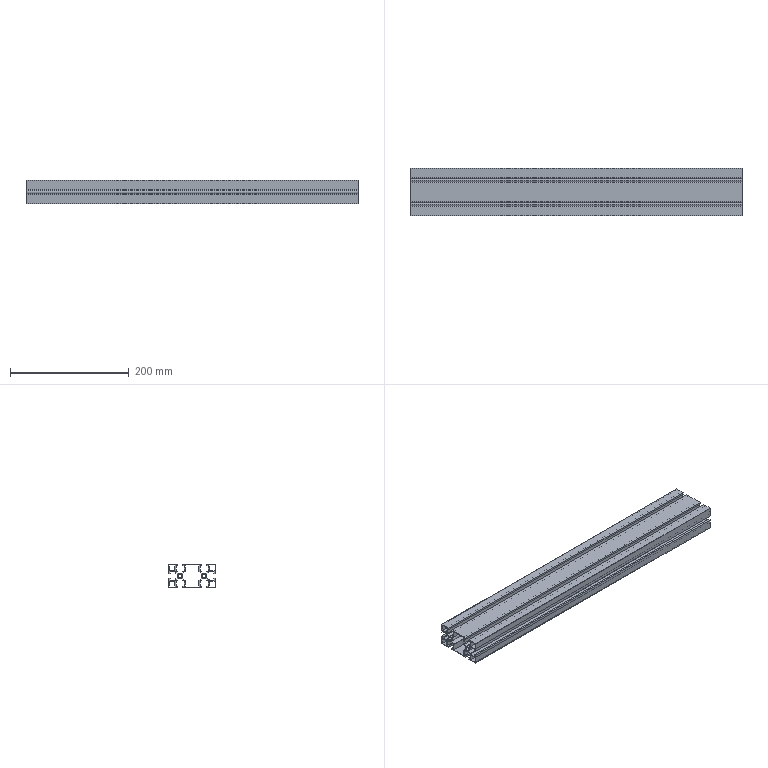Part | 1 solid | 126 faces | box 560 x 80 x 40 mm | volume 388409 mm3 | plane 110 | cylinder 16 | commonest cylinder face diameters 9.6 x10 6.6 x4 0.6 x2